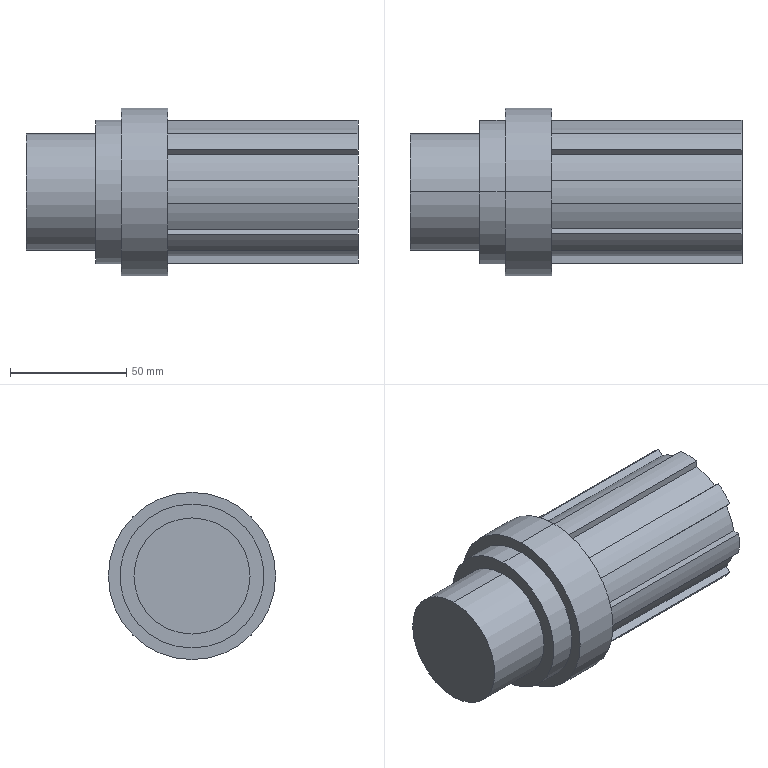Part | SolidWorks | features ICE 2, CirPattern 1, Revolution 1 | 1 solid | 44 faces | box 143 x 72 x 72 mm | volume 395287 mm3 | cylinder 23 | plane 21 | commonest cylinder face diameters 62 x11 56 x8 50 x2 72 x2
STEP:
#1=CARTESIAN_POINT('',(-30.,0.,25.));
#2=VERTEX_POINT('',#1);
#3=CARTESIAN_POINT('',(-30.,0.,-25.));
#4=VERTEX_POINT('',#3);
#5=CARTESIAN_POINT('',(-30.,0.,0.));
#6=DIRECTION('',(-1.,0.,0.));
#7=DIRECTION('',(0.,0.,1.));
#8=AXIS2_PLACEMENT_3D('',#5,#6,#7);
#9=CIRCLE('',#8,25.);
#10=EDGE_CURVE('',#2,#4,#9,.T.);
#11=ORIENTED_EDGE('',*,*,#10,.F.);
#12=CARTESIAN_POINT('',(0.,0.,25.));
#13=VERTEX_POINT('',#12);
#14=CARTESIAN_POINT('',(-30.,0.,25.));
#15=DIRECTION('',(1.,0.,0.));
#16=VECTOR('',#15,1000.);
#17=LINE('',#14,#16);
#18=EDGE_CURVE('',#2,#13,#17,.T.);
#19=ORIENTED_EDGE('',*,*,#18,.T.);
#20=CARTESIAN_POINT('',(0.,0.,-25.));
#21=VERTEX_POINT('',#20);
#22=CARTESIAN_POINT('',(0.,0.,0.));
#23=DIRECTION('',(-1.,0.,0.));
#24=DIRECTION('',(0.,0.,1.));
#25=AXIS2_PLACEMENT_3D('',#22,#23,#24);
#26=CIRCLE('',#25,25.);
#27=EDGE_CURVE('',#13,#21,#26,.T.);
#28=ORIENTED_EDGE('',*,*,#27,.T.);
#29=CARTESIAN_POINT('',(-30.,0.,-25.));
#30=DIRECTION('',(1.,0.,0.));
#31=VECTOR('',#30,1000.);
#32=LINE('',#29,#31);
#33=EDGE_CURVE('',#4,#21,#32,.T.);
#34=ORIENTED_EDGE('',*,*,#33,.F.);
#35=EDGE_LOOP('',(#11,#19,#28,#34));
#36=FACE_OUTER_BOUND('',#35,.T.);
#37=CARTESIAN_POINT('',(-30.,0.,0.));
#38=DIRECTION('',(1.,0.,0.));
#39=DIRECTION('',(0.,0.,-1.));
#40=AXIS2_PLACEMENT_3D('',#37,#38,#39);
#41=CYLINDRICAL_SURFACE('',#40,25.);
#42=ADVANCED_FACE('',(#36),#41,.T.);
#43=CARTESIAN_POINT('',(31.,0.,-31.));
#44=VERTEX_POINT('',#43);
#45=CARTESIAN_POINT('',(31.,-5.,-30.594));
#46=VERTEX_POINT('',#45);
#47=CARTESIAN_POINT('',(31.,0.,0.));
#48=DIRECTION('',(-1.,0.,0.));
#49=DIRECTION('',(0.,0.,-1.));
#50=AXIS2_PLACEMENT_3D('',#47,#48,#49);
#51=CIRCLE('',#50,31.);
#52=EDGE_CURVE('',#44,#46,#51,.T.);
#53=ORIENTED_EDGE('',*,*,#52,.F.);
#54=CARTESIAN_POINT('',(113.,0.,-31.));
#55=VERTEX_POINT('',#54);
#56=CARTESIAN_POINT('',(20.422,0.,-31.));
#57=DIRECTION('',(1.,0.,0.));
#58=VECTOR('',#57,1000.);
#59=LINE('',#56,#58);
#60=EDGE_CURVE('',#44,#55,#59,.T.);
#61=ORIENTED_EDGE('',*,*,#60,.T.);
#62=CARTESIAN_POINT('',(113.,-5.,-30.594));
#63=VERTEX_POINT('',#62);
#64=CARTESIAN_POINT('',(113.,0.,0.));
#65=DIRECTION('',(1.,0.,0.));
#66=DIRECTION('',(0.,-1.,0.));
#67=AXIS2_PLACEMENT_3D('',#64,#65,#66);
#68=CIRCLE('',#67,31.);
#69=EDGE_CURVE('',#63,#55,#68,.T.);
#70=ORIENTED_EDGE('',*,*,#69,.F.);
#71=CARTESIAN_POINT('',(20.422,-5.,-30.594));
#72=DIRECTION('',(1.,0.,0.));
#73=VECTOR('',#72,1000.);
#74=LINE('',#71,#73);
#75=EDGE_CURVE('',#46,#63,#74,.T.);
#76=ORIENTED_EDGE('',*,*,#75,.F.);
#77=EDGE_LOOP('',(#53,#61,#70,#76));
#78=FACE_OUTER_BOUND('',#77,.T.);
#79=CARTESIAN_POINT('',(20.422,0.,0.));
#80=DIRECTION('',(1.,0.,0.));
#81=DIRECTION('',(0.,0.,-1.));
#82=AXIS2_PLACEMENT_3D('',#79,#80,#81);
#83=CYLINDRICAL_SURFACE('',#82,31.);
#84=ADVANCED_FACE('',(#78),#83,.T.);
#85=CARTESIAN_POINT('',(11.,0.,-36.));
#86=VERTEX_POINT('',#85);
#87=CARTESIAN_POINT('',(11.,0.,36.));
#88=VERTEX_POINT('',#87);
#89=CARTESIAN_POINT('',(11.,0.,0.));
#90=DIRECTION('',(1.,0.,0.));
#91=DIRECTION('',(0.,0.,-1.));
#92=AXIS2_PLACEMENT_3D('',#89,#90,#91);
#93=CIRCLE('',#92,36.);
#94=EDGE_CURVE('',#86,#88,#93,.T.);
#95=ORIENTED_EDGE('',*,*,#94,.T.);
#96=CARTESIAN_POINT('',(31.,0.,36.));
#97=VERTEX_POINT('',#96);
#98=CARTESIAN_POINT('',(113.,0.,36.));
#99=DIRECTION('',(1.,0.,0.));
#100=VECTOR('',#99,1000.);
#101=LINE('',#98,#100);
#102=EDGE_CURVE('',#88,#97,#101,.T.);
#103=ORIENTED_EDGE('',*,*,#102,.T.);
#104=CARTESIAN_POINT('',(31.,0.,-36.));
#105=VERTEX_POINT('',#104);
#106=CARTESIAN_POINT('',(31.,0.,0.));
#107=DIRECTION('',(1.,0.,0.));
#108=DIRECTION('',(0.,0.,-1.));
#109=AXIS2_PLACEMENT_3D('',#106,#107,#108);
#110=CIRCLE('',#109,36.);
#111=EDGE_CURVE('',#105,#97,#110,.T.);
#112=ORIENTED_EDGE('',*,*,#111,.F.);
#113=CARTESIAN_POINT('',(113.,0.,-36.));
#114=DIRECTION('',(1.,0.,0.));
#115=VECTOR('',#114,1000.);
#116=LINE('',#113,#115);
#117=EDGE_CURVE('',#86,#105,#116,.T.);
#118=ORIENTED_EDGE('',*,*,#117,.F.);
#119=EDGE_LOOP('',(#95,#103,#112,#118));
#120=FACE_OUTER_BOUND('',#119,.T.);
#121=CARTESIAN_POINT('',(113.,0.,0.));
#122=DIRECTION('',(1.,0.,0.));
#123=DIRECTION('',(0.,0.,-1.));
#124=AXIS2_PLACEMENT_3D('',#121,#122,#123);
#125=CYLINDRICAL_SURFACE('',#124,36.);
#126=ADVANCED_FACE('',(#120),#125,.T.);
#127=CARTESIAN_POINT('',(0.,0.,-31.));
#128=VERTEX_POINT('',#127);
#129=CARTESIAN_POINT('',(0.,0.,31.));
#130=VERTEX_POINT('',#129);
#131=CARTESIAN_POINT('',(0.,0.,0.));
#132=DIRECTION('',(1.,0.,0.));
#133=DIRECTION('',(0.,0.,-1.));
#134=AXIS2_PLACEMENT_3D('',#131,#132,#133);
#135=CIRCLE('',#134,31.);
#136=EDGE_CURVE('',#128,#130,#135,.T.);
#137=ORIENTED_EDGE('',*,*,#136,.T.);
#138=CARTESIAN_POINT('',(11.,0.,31.));
#139=VERTEX_POINT('',#138);
#140=CARTESIAN_POINT('',(113.,0.,31.));
#141=DIRECTION('',(1.,0.,0.));
#142=VECTOR('',#141,1000.);
#143=LINE('',#140,#142);
#144=EDGE_CURVE('',#130,#139,#143,.T.);
#145=ORIENTED_EDGE('',*,*,#144,.T.);
#146=CARTESIAN_POINT('',(11.,0.,-31.));
#147=VERTEX_POINT('',#146);
#148=CARTESIAN_POINT('',(11.,0.,0.));
#149=DIRECTION('',(1.,0.,0.));
#150=DIRECTION('',(0.,0.,-1.));
#151=AXIS2_PLACEMENT_3D('',#148,#149,#150);
#152=CIRCLE('',#151,31.);
#153=EDGE_CURVE('',#147,#139,#152,.T.);
#154=ORIENTED_EDGE('',*,*,#153,.F.);
#155=CARTESIAN_POINT('',(113.,0.,-31.));
#156=DIRECTION('',(1.,0.,0.));
#157=VECTOR('',#156,1000.);
#158=LINE('',#155,#157);
#159=EDGE_CURVE('',#128,#147,#158,.T.);
#160=ORIENTED_EDGE('',*,*,#159,.F.);
#161=EDGE_LOOP('',(#137,#145,#154,#160));
#162=FACE_OUTER_BOUND('',#161,.T.);
#163=CARTESIAN_POINT('',(113.,0.,0.));
#164=DIRECTION('',(1.,0.,0.));
#165=DIRECTION('',(0.,0.,-1.));
#166=AXIS2_PLACEMENT_3D('',#163,#164,#165);
#167=CYLINDRICAL_SURFACE('',#166,31.);
#168=ADVANCED_FACE('',(#162),#167,.T.);
#169=CARTESIAN_POINT('',(31.,23.016,-15.945));
#170=VERTEX_POINT('',#169);
#171=CARTESIAN_POINT('',(113.,23.016,-15.945));
#172=VERTEX_POINT('',#171);
#173=CARTESIAN_POINT('',(17.956,23.016,-15.945));
#174=DIRECTION('',(1.,0.,0.));
#175=VECTOR('',#174,1000.);
#176=LINE('',#173,#175);
#177=EDGE_CURVE('',#170,#172,#176,.T.);
#178=ORIENTED_EDGE('',*,*,#177,.F.);
#179=CARTESIAN_POINT('',(31.,27.55,-5.));
#180=VERTEX_POINT('',#179);
#181=CARTESIAN_POINT('',(31.,0.,0.));
#182=DIRECTION('',(1.,0.,0.));
#183=DIRECTION('',(0.,0.,-1.));
#184=AXIS2_PLACEMENT_3D('',#181,#182,#183);
#185=CIRCLE('',#184,28.);
#186=EDGE_CURVE('',#170,#180,#185,.T.);
#187=ORIENTED_EDGE('',*,*,#186,.T.);
#188=CARTESIAN_POINT('',(113.,27.55,-5.));
#189=VERTEX_POINT('',#188);
#190=CARTESIAN_POINT('',(20.422,27.55,-5.));
#191=DIRECTION('',(1.,0.,0.));
#192=VECTOR('',#191,1000.);
#193=LINE('',#190,#192);
#194=EDGE_CURVE('',#180,#189,#193,.T.);
#195=ORIENTED_EDGE('',*,*,#194,.T.);
#196=CARTESIAN_POINT('',(113.,0.,0.));
#197=DIRECTION('',(1.,0.,0.));
#198=DIRECTION('',(0.,0.,-1.));
#199=AXIS2_PLACEMENT_3D('',#196,#197,#198);
#200=CIRCLE('',#199,28.);
#201=EDGE_CURVE('',#172,#189,#200,.T.);
#202=ORIENTED_EDGE('',*,*,#201,.F.);
#203=EDGE_LOOP('',(#178,#187,#195,#202));
#204=FACE_OUTER_BOUND('',#203,.T.);
#205=CARTESIAN_POINT('',(113.,0.,0.));
#206=DIRECTION('',(1.,0.,0.));
#207=DIRECTION('',(0.,0.,-1.));
#208=AXIS2_PLACEMENT_3D('',#205,#206,#207);
#209=CYLINDRICAL_SURFACE('',#208,28.);
#210=ADVANCED_FACE('',(#204),#209,.T.);
#211=CARTESIAN_POINT('',(31.,15.945,-23.016));
#212=VERTEX_POINT('',#211);
#213=CARTESIAN_POINT('',(113.,15.945,-23.016));
#214=VERTEX_POINT('',#213);
#215=CARTESIAN_POINT('',(17.956,15.945,-23.016));
#216=DIRECTION('',(1.,0.,0.));
#217=VECTOR('',#216,1000.);
#218=LINE('',#215,#217);
#219=EDGE_CURVE('',#212,#214,#218,.T.);
#220=ORIENTED_EDGE('',*,*,#219,.T.);
#221=CARTESIAN_POINT('',(113.,5.,-27.55));
#222=VERTEX_POINT('',#221);
#223=CARTESIAN_POINT('',(113.,0.,0.));
#224=DIRECTION('',(1.,0.,0.));
#225=DIRECTION('',(0.,0.,-1.));
#226=AXIS2_PLACEMENT_3D('',#223,#224,#225);
#227=CIRCLE('',#226,28.);
#228=EDGE_CURVE('',#222,#214,#227,.T.);
#229=ORIENTED_EDGE('',*,*,#228,.F.);
#230=CARTESIAN_POINT('',(31.,5.,-27.55));
#231=VERTEX_POINT('',#230);
#232=CARTESIAN_POINT('',(20.422,5.,-27.55));
#233=DIRECTION('',(1.,0.,0.));
#234=VECTOR('',#233,1000.);
#235=LINE('',#232,#234);
#236=EDGE_CURVE('',#231,#222,#235,.T.);
#237=ORIENTED_EDGE('',*,*,#236,.F.);
#238=CARTESIAN_POINT('',(31.,0.,0.));
#239=DIRECTION('',(1.,0.,0.));
#240=DIRECTION('',(0.,0.,-1.));
#241=AXIS2_PLACEMENT_3D('',#238,#239,#240);
#242=CIRCLE('',#241,28.);
#243=EDGE_CURVE('',#231,#212,#242,.T.);
#244=ORIENTED_EDGE('',*,*,#243,.T.);
#245=EDGE_LOOP('',(#220,#229,#237,#244));
#246=FACE_OUTER_BOUND('',#245,.T.);
#247=CARTESIAN_POINT('',(113.,0.,0.));
#248=DIRECTION('',(1.,0.,0.));
#249=DIRECTION('',(0.,0.,-1.));
#250=AXIS2_PLACEMENT_3D('',#247,#248,#249);
#251=CYLINDRICAL_SURFACE('',#250,28.);
#252=ADVANCED_FACE('',(#246),#251,.T.);
#253=CARTESIAN_POINT('',(31.,-5.,-27.55));
#254=VERTEX_POINT('',#253);
#255=CARTESIAN_POINT('',(113.,-5.,-27.55));
#256=VERTEX_POINT('',#255);
#257=CARTESIAN_POINT('',(20.422,-5.,-27.55));
#258=DIRECTION('',(1.,0.,0.));
#259=VECTOR('',#258,1000.);
#260=LINE('',#257,#259);
#261=EDGE_CURVE('',#254,#256,#260,.T.);
#262=ORIENTED_EDGE('',*,*,#261,.T.);
#263=CARTESIAN_POINT('',(113.,-15.945,-23.016));
#264=VERTEX_POINT('',#263);
#265=CARTESIAN_POINT('',(113.,0.,0.));
#266=DIRECTION('',(1.,0.,0.));
#267=DIRECTION('',(0.,0.,-1.));
#268=AXIS2_PLACEMENT_3D('',#265,#266,#267);
#269=CIRCLE('',#268,28.);
#270=EDGE_CURVE('',#264,#256,#269,.T.);
#271=ORIENTED_EDGE('',*,*,#270,.F.);
#272=CARTESIAN_POINT('',(31.,-15.945,-23.016));
#273=VERTEX_POINT('',#272);
#274=CARTESIAN_POINT('',(17.956,-15.945,-23.016));
#275=DIRECTION('',(1.,0.,0.));
#276=VECTOR('',#275,1000.);
#277=LINE('',#274,#276);
#278=EDGE_CURVE('',#273,#264,#277,.T.);
#279=ORIENTED_EDGE('',*,*,#278,.F.);
#280=CARTESIAN_POINT('',(31.,0.,0.));
#281=DIRECTION('',(1.,0.,0.));
#282=DIRECTION('',(0.,0.,-1.));
#283=AXIS2_PLACEMENT_3D('',#280,#281,#282);
#284=CIRCLE('',#283,28.);
#285=EDGE_CURVE('',#273,#254,#284,.T.);
#286=ORIENTED_EDGE('',*,*,#285,.T.);
#287=EDGE_LOOP('',(#262,#271,#279,#286));
#288=FACE_OUTER_BOUND('',#287,.T.);
#289=CARTESIAN_POINT('',(113.,0.,0.));
#290=DIRECTION('',(1.,0.,0.));
#291=DIRECTION('',(0.,0.,-1.));
#292=AXIS2_PLACEMENT_3D('',#289,#290,#291);
#293=CYLINDRICAL_SURFACE('',#292,28.);
#294=ADVANCED_FACE('',(#288),#293,.T.);
#295=CARTESIAN_POINT('',(31.,-23.016,-15.945));
#296=VERTEX_POINT('',#295);
#297=CARTESIAN_POINT('',(113.,-23.016,-15.945));
#298=VERTEX_POINT('',#297);
#299=CARTESIAN_POINT('',(17.956,-23.016,-15.945));
#300=DIRECTION('',(1.,0.,0.));
#301=VECTOR('',#300,1000.);
#302=LINE('',#299,#301);
#303=EDGE_CURVE('',#296,#298,#302,.T.);
#304=ORIENTED_EDGE('',*,*,#303,.T.);
#305=CARTESIAN_POINT('',(113.,-27.55,-5.));
#306=VERTEX_POINT('',#305);
#307=CARTESIAN_POINT('',(113.,0.,0.));
#308=DIRECTION('',(1.,0.,0.));
#309=DIRECTION('',(0.,0.,-1.));
#310=AXIS2_PLACEMENT_3D('',#307,#308,#309);
#311=CIRCLE('',#310,28.);
#312=EDGE_CURVE('',#306,#298,#311,.T.);
#313=ORIENTED_EDGE('',*,*,#312,.F.);
#314=CARTESIAN_POINT('',(31.,-27.55,-5.));
#315=VERTEX_POINT('',#314);
#316=CARTESIAN_POINT('',(20.422,-27.55,-5.));
#317=DIRECTION('',(1.,0.,0.));
#318=VECTOR('',#317,1000.);
#319=LINE('',#316,#318);
#320=EDGE_CURVE('',#315,#306,#319,.T.);
#321=ORIENTED_EDGE('',*,*,#320,.F.);
#322=CARTESIAN_POINT('',(31.,0.,0.));
#323=DIRECTION('',(1.,0.,0.));
#324=DIRECTION('',(0.,0.,-1.));
#325=AXIS2_PLACEMENT_3D('',#322,#323,#324);
#326=CIRCLE('',#325,28.);
#327=EDGE_CURVE('',#315,#296,#326,.T.);
#328=ORIENTED_EDGE('',*,*,#327,.T.);
#329=EDGE_LOOP('',(#304,#313,#321,#328));
#330=FACE_OUTER_BOUND('',#329,.T.);
#331=CARTESIAN_POINT('',(113.,0.,0.));
#332=DIRECTION('',(1.,0.,0.));
#333=DIRECTION('',(0.,0.,-1.));
#334=AXIS2_PLACEMENT_3D('',#331,#332,#333);
#335=CYLINDRICAL_SURFACE('',#334,28.);
#336=ADVANCED_FACE('',(#330),#335,.T.);
#337=CARTESIAN_POINT('',(31.,-27.55,5.));
#338=VERTEX_POINT('',#337);
#339=CARTESIAN_POINT('',(113.,-27.55,5.));
#340=VERTEX_POINT('',#339);
#341=CARTESIAN_POINT('',(20.422,-27.55,5.));
#342=DIRECTION('',(1.,0.,0.));
#343=VECTOR('',#342,1000.);
#344=LINE('',#341,#343);
#345=EDGE_CURVE('',#338,#340,#344,.T.);
#346=ORIENTED_EDGE('',*,*,#345,.T.);
#347=CARTESIAN_POINT('',(113.,-23.016,15.945));
#348=VERTEX_POINT('',#347);
#349=CARTESIAN_POINT('',(113.,0.,0.));
#350=DIRECTION('',(1.,0.,0.));
#351=DIRECTION('',(0.,0.,-1.));
#352=AXIS2_PLACEMENT_3D('',#349,#350,#351);
#353=CIRCLE('',#352,28.);
#354=EDGE_CURVE('',#348,#340,#353,.T.);
#355=ORIENTED_EDGE('',*,*,#354,.F.);
#356=CARTESIAN_POINT('',(31.,-23.016,15.945));
#357=VERTEX_POINT('',#356);
#358=CARTESIAN_POINT('',(17.956,-23.016,15.945));
#359=DIRECTION('',(1.,0.,0.));
#360=VECTOR('',#359,1000.);
#361=LINE('',#358,#360);
#362=EDGE_CURVE('',#357,#348,#361,.T.);
#363=ORIENTED_EDGE('',*,*,#362,.F.);
#364=CARTESIAN_POINT('',(31.,0.,0.));
#365=DIRECTION('',(1.,0.,0.));
#366=DIRECTION('',(0.,0.,-1.));
#367=AXIS2_PLACEMENT_3D('',#364,#365,#366);
#368=CIRCLE('',#367,28.);
#369=EDGE_CURVE('',#357,#338,#368,.T.);
#370=ORIENTED_EDGE('',*,*,#369,.T.);
#371=EDGE_LOOP('',(#346,#355,#363,#370));
#372=FACE_OUTER_BOUND('',#371,.T.);
#373=CARTESIAN_POINT('',(113.,0.,0.));
#374=DIRECTION('',(1.,0.,0.));
#375=DIRECTION('',(0.,0.,-1.));
#376=AXIS2_PLACEMENT_3D('',#373,#374,#375);
#377=CYLINDRICAL_SURFACE('',#376,28.);
#378=ADVANCED_FACE('',(#372),#377,.T.);
#379=CARTESIAN_POINT('',(31.,-15.945,23.016));
#380=VERTEX_POINT('',#379);
#381=CARTESIAN_POINT('',(113.,-15.945,23.016));
#382=VERTEX_POINT('',#381);
#383=CARTESIAN_POINT('',(17.956,-15.945,23.016));
#384=DIRECTION('',(1.,0.,0.));
#385=VECTOR('',#384,1000.);
#386=LINE('',#383,#385);
#387=EDGE_CURVE('',#380,#382,#386,.T.);
#388=ORIENTED_EDGE('',*,*,#387,.T.);
#389=CARTESIAN_POINT('',(113.,-5.,27.55));
#390=VERTEX_POINT('',#389);
#391=CARTESIAN_POINT('',(113.,0.,0.));
#392=DIRECTION('',(1.,0.,0.));
#393=DIRECTION('',(0.,0.,-1.));
#394=AXIS2_PLACEMENT_3D('',#391,#392,#393);
#395=CIRCLE('',#394,28.);
#396=EDGE_CURVE('',#390,#382,#395,.T.);
#397=ORIENTED_EDGE('',*,*,#396,.F.);
#398=CARTESIAN_POINT('',(31.,-5.,27.55));
#399=VERTEX_POINT('',#398);
#400=CARTESIAN_POINT('',(20.422,-5.,27.55));
#401=DIRECTION('',(1.,0.,0.));
#402=VECTOR('',#401,1000.);
#403=LINE('',#400,#402);
#404=EDGE_CURVE('',#399,#390,#403,.T.);
#405=ORIENTED_EDGE('',*,*,#404,.F.);
#406=CARTESIAN_POINT('',(31.,0.,0.));
#407=DIRECTION('',(1.,0.,0.));
#408=DIRECTION('',(0.,0.,-1.));
#409=AXIS2_PLACEMENT_3D('',#406,#407,#408);
#410=CIRCLE('',#409,28.);
#411=EDGE_CURVE('',#399,#380,#410,.T.);
#412=ORIENTED_EDGE('',*,*,#411,.T.);
#413=EDGE_LOOP('',(#388,#397,#405,#412));
#414=FACE_OUTER_BOUND('',#413,.T.);
#415=CARTESIAN_POINT('',(113.,0.,0.));
#416=DIRECTION('',(1.,0.,0.));
#417=DIRECTION('',(0.,0.,-1.));
#418=AXIS2_PLACEMENT_3D('',#415,#416,#417);
#419=CYLINDRICAL_SURFACE('',#418,28.);
#420=ADVANCED_FACE('',(#414),#419,.T.);
#421=CARTESIAN_POINT('',(31.,5.,27.55));
#422=VERTEX_POINT('',#421);
#423=CARTESIAN_POINT('',(113.,5.,27.55));
#424=VERTEX_POINT('',#423);
#425=CARTESIAN_POINT('',(20.422,5.,27.55));
#426=DIRECTION('',(1.,0.,0.));
#427=VECTOR('',#426,1000.);
#428=LINE('',#425,#427);
#429=EDGE_CURVE('',#422,#424,#428,.T.);
#430=ORIENTED_EDGE('',*,*,#429,.T.);
#431=CARTESIAN_POINT('',(113.,15.945,23.016));
#432=VERTEX_POINT('',#431);
#433=CARTESIAN_POINT('',(113.,0.,0.));
#434=DIRECTION('',(1.,0.,0.));
#435=DIRECTION('',(0.,0.,-1.));
#436=AXIS2_PLACEMENT_3D('',#433,#434,#435);
#437=CIRCLE('',#436,28.);
#438=EDGE_CURVE('',#432,#424,#437,.T.);
#439=ORIENTED_EDGE('',*,*,#438,.F.);
#440=CARTESIAN_POINT('',(31.,15.945,23.016));
#441=VERTEX_POINT('',#440);
#442=CARTESIAN_POINT('',(17.956,15.945,23.016));
#443=DIRECTION('',(1.,0.,0.));
#444=VECTOR('',#443,1000.);
#445=LINE('',#442,#444);
#446=EDGE_CURVE('',#441,#432,#445,.T.);
#447=ORIENTED_EDGE('',*,*,#446,.F.);
#448=CARTESIAN_POINT('',(31.,0.,0.));
#449=DIRECTION('',(1.,0.,0.));
#450=DIRECTION('',(0.,0.,-1.));
#451=AXIS2_PLACEMENT_3D('',#448,#449,#450);
#452=CIRCLE('',#451,28.);
#453=EDGE_CURVE('',#441,#422,#452,.T.);
#454=ORIENTED_EDGE('',*,*,#453,.T.);
#455=EDGE_LOOP('',(#430,#439,#447,#454));
#456=FACE_OUTER_BOUND('',#455,.T.);
#457=CARTESIAN_POINT('',(113.,0.,0.));
#458=DIRECTION('',(1.,0.,0.));
#459=DIRECTION('',(0.,0.,-1.));
#460=AXIS2_PLACEMENT_3D('',#457,#458,#459);
#461=CYLINDRICAL_SURFACE('',#460,28.);
#462=ADVANCED_FACE('',(#456),#461,.T.);
#463=CARTESIAN_POINT('',(0.,0.,0.));
#464=DIRECTION('',(-1.,0.,0.));
#465=DIRECTION('',(0.,0.,1.));
#466=AXIS2_PLACEMENT_3D('',#463,#464,#465);
#467=CIRCLE('',#466,25.);
#468=EDGE_CURVE('',#21,#13,#467,.T.);
#469=ORIENTED_EDGE('',*,*,#468,.F.);
#470=ORIENTED_EDGE('',*,*,#27,.F.);
#471=EDGE_LOOP('',(#469,#470));
#472=FACE_BOUND('',#471,.T.);
#473=ORIENTED_EDGE('',*,*,#136,.F.);
#474=CARTESIAN_POINT('',(0.,0.,0.));
#475=DIRECTION('',(1.,0.,0.));
#476=DIRECTION('',(0.,0.,-1.));
#477=AXIS2_PLACEMENT_3D('',#474,#475,#476);
#478=CIRCLE('',#477,31.);
#479=EDGE_CURVE('',#130,#128,#478,.T.);
#480=ORIENTED_EDGE('',*,*,#479,.F.);
#481=EDGE_LOOP('',(#473,#480));
#482=FACE_OUTER_BOUND('',#481,.T.);
#483=CARTESIAN_POINT('',(0.,0.,0.));
#484=DIRECTION('',(-1.,0.,0.));
#485=DIRECTION('',(0.,0.,1.));
#486=AXIS2_PLACEMENT_3D('',#483,#484,#485);
#487=PLANE('',#486);
#488=ADVANCED_FACE('',(#472,#482),#487,.T.);
#489=ORIENTED_EDGE('',*,*,#144,.F.);
#490=ORIENTED_EDGE('',*,*,#479,.T.);
#491=ORIENTED_EDGE('',*,*,#159,.T.);
#492=CARTESIAN_POINT('',(11.,0.,0.));
#493=DIRECTION('',(1.,0.,0.));
#494=DIRECTION('',(0.,0.,-1.));
#495=AXIS2_PLACEMENT_3D('',#492,#493,#494);
#496=CIRCLE('',#495,31.);
#497=EDGE_CURVE('',#139,#147,#496,.T.);
#498=ORIENTED_EDGE('',*,*,#497,.F.);
#499=EDGE_LOOP('',(#489,#490,#491,#498));
#500=FACE_OUTER_BOUND('',#499,.T.);
#501=CARTESIAN_POINT('',(113.,0.,0.));
#502=DIRECTION('',(1.,0.,0.));
#503=DIRECTION('',(0.,0.,-1.));
#504=AXIS2_PLACEMENT_3D('',#501,#502,#503);
#505=CYLINDRICAL_SURFACE('',#504,31.);
#506=ADVANCED_FACE('',(#500),#505,.T.);
#507=ORIENTED_EDGE('',*,*,#153,.T.);
#508=ORIENTED_EDGE('',*,*,#497,.T.);
#509=EDGE_LOOP('',(#507,#508));
#510=FACE_BOUND('',#509,.T.);
#511=ORIENTED_EDGE('',*,*,#94,.F.);
#512=CARTESIAN_POINT('',(11.,0.,0.));
#513=DIRECTION('',(1.,0.,0.));
#514=DIRECTION('',(0.,0.,-1.));
#515=AXIS2_PLACEMENT_3D('',#512,#513,#514);
#516=CIRCLE('',#515,36.);
#517=EDGE_CURVE('',#88,#86,#516,.T.);
#518=ORIENTED_EDGE('',*,*,#517,.F.);
#519=EDGE_LOOP('',(#511,#518));
#520=FACE_OUTER_BOUND('',#519,.T.);
#521=CARTESIAN_POINT('',(11.,0.,-31.));
#522=DIRECTION('',(-1.,0.,0.));
#523=DIRECTION('',(0.,0.,1.));
#524=AXIS2_PLACEMENT_3D('',#521,#522,#523);
#525=PLANE('',#524);
#526=ADVANCED_FACE('',(#510,#520),#525,.T.);
#527=ORIENTED_EDGE('',*,*,#102,.F.);
#528=ORIENTED_EDGE('',*,*,#517,.T.);
#529=ORIENTED_EDGE('',*,*,#117,.T.);
#530=CARTESIAN_POINT('',(31.,0.,0.));
#531=DIRECTION('',(1.,0.,0.));
#532=DIRECTION('',(0.,0.,-1.));
#533=AXIS2_PLACEMENT_3D('',#530,#531,#532);
#534=CIRCLE('',#533,36.);
#535=EDGE_CURVE('',#97,#105,#534,.T.);
#536=ORIENTED_EDGE('',*,*,#535,.F.);
#537=EDGE_LOOP('',(#527,#528,#529,#536));
#538=FACE_OUTER_BOUND('',#537,.T.);
#539=CARTESIAN_POINT('',(113.,0.,0.));
#540=DIRECTION('',(1.,0.,0.));
#541=DIRECTION('',(0.,0.,-1.));
#542=AXIS2_PLACEMENT_3D('',#539,#540,#541);
#543=CYLINDRICAL_SURFACE('',#542,36.);
#544=ADVANCED_FACE('',(#538),#543,.T.);
#545=CARTESIAN_POINT('',(31.,25.169,-18.098));
#546=VERTEX_POINT('',#545);
#547=CARTESIAN_POINT('',(31.,25.169,-18.098));
#548=DIRECTION('',(0.,0.7071,-0.7071));
#549=VECTOR('',#548,1000.);
#550=LINE('',#547,#549);
#551=EDGE_CURVE('',#170,#546,#550,.T.);
#552=ORIENTED_EDGE('',*,*,#551,.T.);
#553=CARTESIAN_POINT('',(31.,18.098,-25.169));
#554=VERTEX_POINT('',#553);
#555=CARTESIAN_POINT('',(31.,0.,0.));
#556=DIRECTION('',(-1.,0.,0.));
#557=DIRECTION('',(0.,0.,-1.));
#558=AXIS2_PLACEMENT_3D('',#555,#556,#557);
#559=CIRCLE('',#558,31.);
#560=EDGE_CURVE('',#546,#554,#559,.T.);
#561=ORIENTED_EDGE('',*,*,#560,.T.);
#562=CARTESIAN_POINT('',(31.,18.098,-25.169));
#563=DIRECTION('',(0.,-0.7071,0.7071));
#564=VECTOR('',#563,1000.);
#565=LINE('',#562,#564);
#566=EDGE_CURVE('',#554,#212,#565,.T.);
#567=ORIENTED_EDGE('',*,*,#566,.T.);
#568=ORIENTED_EDGE('',*,*,#243,.F.);
#569=CARTESIAN_POINT('',(31.,5.,-30.594));
#570=VERTEX_POINT('',#569);
#571=CARTESIAN_POINT('',(31.,5.,-30.594));
#572=DIRECTION('',(0.,0.,-1.));
#573=VECTOR('',#572,1000.);
#574=LINE('',#571,#573);
#575=EDGE_CURVE('',#231,#570,#574,.T.);
#576=ORIENTED_EDGE('',*,*,#575,.T.);
#577=CARTESIAN_POINT('',(31.,0.,0.));
#578=DIRECTION('',(-1.,0.,0.));
#579=DIRECTION('',(0.,0.,-1.));
#580=AXIS2_PLACEMENT_3D('',#577,#578,#579);
#581=CIRCLE('',#580,31.);
#582=EDGE_CURVE('',#570,#44,#581,.T.);
#583=ORIENTED_EDGE('',*,*,#582,.T.);
#584=ORIENTED_EDGE('',*,*,#52,.T.);
#585=CARTESIAN_POINT('',(31.,-5.,-30.594));
#586=DIRECTION('',(0.,0.,1.));
#587=VECTOR('',#586,1000.);
#588=LINE('',#585,#587);
#589=EDGE_CURVE('',#46,#254,#588,.T.);
#590=ORIENTED_EDGE('',*,*,#589,.T.);
#591=ORIENTED_EDGE('',*,*,#285,.F.);
#592=CARTESIAN_POINT('',(31.,-18.098,-25.169));
#593=VERTEX_POINT('',#592);
#594=CARTESIAN_POINT('',(31.,-18.098,-25.169));
#595=DIRECTION('',(0.,-0.7071,-0.7071));
#596=VECTOR('',#595,1000.);
#597=LINE('',#594,#596);
#598=EDGE_CURVE('',#273,#593,#597,.T.);
#599=ORIENTED_EDGE('',*,*,#598,.T.);
#600=CARTESIAN_POINT('',(31.,-25.169,-18.098));
#601=VERTEX_POINT('',#600);
#602=CARTESIAN_POINT('',(31.,0.,0.));
#603=DIRECTION('',(-1.,0.,0.));
#604=DIRECTION('',(0.,0.,-1.));
#605=AXIS2_PLACEMENT_3D('',#602,#603,#604);
#606=CIRCLE('',#605,31.);
#607=EDGE_CURVE('',#593,#601,#606,.T.);
#608=ORIENTED_EDGE('',*,*,#607,.T.);
#609=CARTESIAN_POINT('',(31.,-25.169,-18.098));
#610=DIRECTION('',(0.,0.7071,0.7071));
#611=VECTOR('',#610,1000.);
#612=LINE('',#609,#611);
#613=EDGE_CURVE('',#601,#296,#612,.T.);
#614=ORIENTED_EDGE('',*,*,#613,.T.);
#615=ORIENTED_EDGE('',*,*,#327,.F.);
#616=CARTESIAN_POINT('',(31.,-30.594,-5.));
#617=VERTEX_POINT('',#616);
#618=CARTESIAN_POINT('',(31.,-30.594,-5.));
#619=DIRECTION('',(0.,-1.,0.));
#620=VECTOR('',#619,1000.);
#621=LINE('',#618,#620);
#622=EDGE_CURVE('',#315,#617,#621,.T.);
#623=ORIENTED_EDGE('',*,*,#622,.T.);
#624=CARTESIAN_POINT('',(31.,-30.594,5.));
#625=VERTEX_POINT('',#624);
#626=CARTESIAN_POINT('',(31.,0.,0.));
#627=DIRECTION('',(-1.,0.,0.));
#628=DIRECTION('',(0.,0.,-1.));
#629=AXIS2_PLACEMENT_3D('',#626,#627,#628);
#630=CIRCLE('',#629,31.);
#631=EDGE_CURVE('',#617,#625,#630,.T.);
#632=ORIENTED_EDGE('',*,*,#631,.T.);
#633=CARTESIAN_POINT('',(31.,-30.594,5.));
#634=DIRECTION('',(0.,1.,0.));
#635=VECTOR('',#634,1000.);
#636=LINE('',#633,#635);
#637=EDGE_CURVE('',#625,#338,#636,.T.);
#638=ORIENTED_EDGE('',*,*,#637,.T.);
#639=ORIENTED_EDGE('',*,*,#369,.F.);
#640=CARTESIAN_POINT('',(31.,-25.169,18.098));
#641=VERTEX_POINT('',#640);
#642=CARTESIAN_POINT('',(31.,-25.169,18.098));
#643=DIRECTION('',(0.,-0.7071,0.7071));
#644=VECTOR('',#643,1000.);
#645=LINE('',#642,#644);
#646=EDGE_CURVE('',#357,#641,#645,.T.);
#647=ORIENTED_EDGE('',*,*,#646,.T.);
#648=CARTESIAN_POINT('',(31.,-18.098,25.169));
#649=VERTEX_POINT('',#648);
#650=CARTESIAN_POINT('',(31.,0.,0.));
#651=DIRECTION('',(-1.,0.,0.));
#652=DIRECTION('',(0.,0.,-1.));
#653=AXIS2_PLACEMENT_3D('',#650,#651,#652);
#654=CIRCLE('',#653,31.);
#655=EDGE_CURVE('',#641,#649,#654,.T.);
#656=ORIENTED_EDGE('',*,*,#655,.T.);
#657=CARTESIAN_POINT('',(31.,-18.098,25.169));
#658=DIRECTION('',(0.,0.7071,-0.7071));
#659=VECTOR('',#658,1000.);
#660=LINE('',#657,#659);
#661=EDGE_CURVE('',#649,#380,#660,.T.);
#662=ORIENTED_EDGE('',*,*,#661,.T.);
#663=ORIENTED_EDGE('',*,*,#411,.F.);
#664=CARTESIAN_POINT('',(31.,-5.,30.594));
#665=VERTEX_POINT('',#664);
#666=CARTESIAN_POINT('',(31.,-5.,30.594));
#667=DIRECTION('',(0.,0.,1.));
#668=VECTOR('',#667,1000.);
#669=LINE('',#666,#668);
#670=EDGE_CURVE('',#399,#665,#669,.T.);
#671=ORIENTED_EDGE('',*,*,#670,.T.);
#672=CARTESIAN_POINT('',(31.,5.,30.594));
#673=VERTEX_POINT('',#672);
#674=CARTESIAN_POINT('',(31.,0.,0.));
#675=DIRECTION('',(-1.,0.,0.));
#676=DIRECTION('',(0.,0.,-1.));
#677=AXIS2_PLACEMENT_3D('',#674,#675,#676);
#678=CIRCLE('',#677,31.);
#679=EDGE_CURVE('',#665,#673,#678,.T.);
#680=ORIENTED_EDGE('',*,*,#679,.T.);
#681=CARTESIAN_POINT('',(31.,5.,30.594));
#682=DIRECTION('',(0.,0.,-1.));
#683=VECTOR('',#682,1000.);
#684=LINE('',#681,#683);
#685=EDGE_CURVE('',#673,#422,#684,.T.);
#686=ORIENTED_EDGE('',*,*,#685,.T.);
#687=ORIENTED_EDGE('',*,*,#453,.F.);
#688=CARTESIAN_POINT('',(31.,18.098,25.169));
#689=VERTEX_POINT('',#688);
#690=CARTESIAN_POINT('',(31.,18.098,25.169));
#691=DIRECTION('',(0.,0.7071,0.7071));
#692=VECTOR('',#691,1000.);
#693=LINE('',#690,#692);
#694=EDGE_CURVE('',#441,#689,#693,.T.);
#695=ORIENTED_EDGE('',*,*,#694,.T.);
#696=CARTESIAN_POINT('',(31.,25.169,18.098));
#697=VERTEX_POINT('',#696);
#698=CARTESIAN_POINT('',(31.,0.,0.));
#699=DIRECTION('',(-1.,0.,0.));
#700=DIRECTION('',(0.,0.,-1.));
#701=AXIS2_PLACEMENT_3D('',#698,#699,#700);
#702=CIRCLE('',#701,31.);
#703=EDGE_CURVE('',#689,#697,#702,.T.);
#704=ORIENTED_EDGE('',*,*,#703,.T.);
#705=CARTESIAN_POINT('',(31.,23.016,15.945));
#706=VERTEX_POINT('',#705);
#707=CARTESIAN_POINT('',(31.,25.169,18.098));
#708=DIRECTION('',(0.,-0.7071,-0.7071));
#709=VECTOR('',#708,1000.);
#710=LINE('',#707,#709);
#711=EDGE_CURVE('',#697,#706,#710,.T.);
#712=ORIENTED_EDGE('',*,*,#711,.T.);
#713=CARTESIAN_POINT('',(31.,27.55,5.));
#714=VERTEX_POINT('',#713);
#715=CARTESIAN_POINT('',(31.,0.,0.));
#716=DIRECTION('',(1.,0.,0.));
#717=DIRECTION('',(0.,0.,-1.));
#718=AXIS2_PLACEMENT_3D('',#715,#716,#717);
#719=CIRCLE('',#718,28.);
#720=EDGE_CURVE('',#714,#706,#719,.T.);
#721=ORIENTED_EDGE('',*,*,#720,.F.);
#722=CARTESIAN_POINT('',(31.,30.594,5.));
#723=VERTEX_POINT('',#722);
#724=CARTESIAN_POINT('',(31.,30.594,5.));
#725=DIRECTION('',(0.,1.,0.));
#726=VECTOR('',#725,1000.);
#727=LINE('',#724,#726);
#728=EDGE_CURVE('',#714,#723,#727,.T.);
#729=ORIENTED_EDGE('',*,*,#728,.T.);
#730=CARTESIAN_POINT('',(31.,30.594,-5.));
#731=VERTEX_POINT('',#730);
#732=CARTESIAN_POINT('',(31.,0.,0.));
#733=DIRECTION('',(-1.,0.,0.));
#734=DIRECTION('',(0.,0.,-1.));
#735=AXIS2_PLACEMENT_3D('',#732,#733,#734);
#736=CIRCLE('',#735,31.);
#737=EDGE_CURVE('',#723,#731,#736,.T.);
#738=ORIENTED_EDGE('',*,*,#737,.T.);
#739=CARTESIAN_POINT('',(31.,30.594,-5.));
#740=DIRECTION('',(0.,-1.,0.));
#741=VECTOR('',#740,1000.);
#742=LINE('',#739,#741);
#743=EDGE_CURVE('',#731,#180,#742,.T.);
#744=ORIENTED_EDGE('',*,*,#743,.T.);
#745=ORIENTED_EDGE('',*,*,#186,.F.);
#746=EDGE_LOOP('',(#552,#561,#567,#568,#576,#583,#584,#590,#591,#599,#608,#614,#615,#623,#632,#638,#639,#647,#656,#662,#663,#671,#680,#686,#687,#695,#704,#712,#721,#729,#738,#744,#745));
#747=FACE_BOUND('',#746,.T.);
#748=ORIENTED_EDGE('',*,*,#111,.T.);
#749=ORIENTED_EDGE('',*,*,#535,.T.);
#750=EDGE_LOOP('',(#748,#749));
#751=FACE_OUTER_BOUND('',#750,.T.);
#752=CARTESIAN_POINT('',(31.,0.,-36.));
#753=DIRECTION('',(1.,0.,0.));
#754=DIRECTION('',(0.,0.,-1.));
#755=AXIS2_PLACEMENT_3D('',#752,#753,#754);
#756=PLANE('',#755);
#757=ADVANCED_FACE('',(#747,#751),#756,.T.);
#758=CARTESIAN_POINT('',(113.,23.016,15.945));
#759=VERTEX_POINT('',#758);
#760=CARTESIAN_POINT('',(17.956,23.016,15.945));
#761=DIRECTION('',(1.,0.,0.));
#762=VECTOR('',#761,1000.);
#763=LINE('',#760,#762);
#764=EDGE_CURVE('',#706,#759,#763,.T.);
#765=ORIENTED_EDGE('',*,*,#764,.T.);
#766=CARTESIAN_POINT('',(113.,27.55,5.));
#767=VERTEX_POINT('',#766);
#768=CARTESIAN_POINT('',(113.,0.,0.));
#769=DIRECTION('',(1.,0.,0.));
#770=DIRECTION('',(0.,0.,-1.));
#771=AXIS2_PLACEMENT_3D('',#768,#769,#770);
#772=CIRCLE('',#771,28.);
#773=EDGE_CURVE('',#767,#759,#772,.T.);
#774=ORIENTED_EDGE('',*,*,#773,.F.);
#775=CARTESIAN_POINT('',(20.422,27.55,5.));
#776=DIRECTION('',(1.,0.,0.));
#777=VECTOR('',#776,1000.);
#778=LINE('',#775,#777);
#779=EDGE_CURVE('',#714,#767,#778,.T.);
#780=ORIENTED_EDGE('',*,*,#779,.F.);
#781=ORIENTED_EDGE('',*,*,#720,.T.);
#782=EDGE_LOOP('',(#765,#774,#780,#781));
#783=FACE_OUTER_BOUND('',#782,.T.);
#784=CARTESIAN_POINT('',(113.,0.,0.));
#785=DIRECTION('',(1.,0.,0.));
#786=DIRECTION('',(0.,0.,-1.));
#787=AXIS2_PLACEMENT_3D('',#784,#785,#786);
#788=CYLINDRICAL_SURFACE('',#787,28.);
#789=ADVANCED_FACE('',(#783),#788,.T.);
#790=ORIENTED_EDGE('',*,*,#773,.T.);
#791=CARTESIAN_POINT('',(113.,25.169,18.098));
#792=VERTEX_POINT('',#791);
#793=CARTESIAN_POINT('',(113.,25.169,18.098));
#794=DIRECTION('',(0.,0.7071,0.7071));
#795=VECTOR('',#794,1000.);
#796=LINE('',#793,#795);
#797=EDGE_CURVE('',#759,#792,#796,.T.);
#798=ORIENTED_EDGE('',*,*,#797,.T.);
#799=CARTESIAN_POINT('',(113.,18.098,25.169));
#800=VERTEX_POINT('',#799);
#801=CARTESIAN_POINT('',(113.,0.,0.));
#802=DIRECTION('',(1.,0.,0.));
#803=DIRECTION('',(0.,0.7071,-0.7071));
#804=AXIS2_PLACEMENT_3D('',#801,#802,#803);
#805=CIRCLE('',#804,31.);
#806=EDGE_CURVE('',#792,#800,#805,.T.);
#807=ORIENTED_EDGE('',*,*,#806,.T.);
#808=CARTESIAN_POINT('',(113.,18.098,25.169));
#809=DIRECTION('',(0.,-0.7071,-0.7071));
#810=VECTOR('',#809,1000.);
#811=LINE('',#808,#810);
#812=EDGE_CURVE('',#800,#432,#811,.T.);
#813=ORIENTED_EDGE('',*,*,#812,.T.);
#814=ORIENTED_EDGE('',*,*,#438,.T.);
#815=CARTESIAN_POINT('',(113.,5.,30.594));
#816=VERTEX_POINT('',#815);
#817=CARTESIAN_POINT('',(113.,5.,30.594));
#818=DIRECTION('',(0.,0.,1.));
#819=VECTOR('',#818,1000.);
#820=LINE('',#817,#819);
#821=EDGE_CURVE('',#424,#816,#820,.T.);
#822=ORIENTED_EDGE('',*,*,#821,.T.);
#823=CARTESIAN_POINT('',(113.,-5.,30.594));
#824=VERTEX_POINT('',#823);
#825=CARTESIAN_POINT('',(113.,0.,0.));
#826=DIRECTION('',(1.,0.,0.));
#827=DIRECTION('',(0.,1.,0.));
#828=AXIS2_PLACEMENT_3D('',#825,#826,#827);
#829=CIRCLE('',#828,31.);
#830=EDGE_CURVE('',#816,#824,#829,.T.);
#831=ORIENTED_EDGE('',*,*,#830,.T.);
#832=CARTESIAN_POINT('',(113.,-5.,30.594));
#833=DIRECTION('',(0.,0.,-1.));
#834=VECTOR('',#833,1000.);
#835=LINE('',#832,#834);
#836=EDGE_CURVE('',#824,#390,#835,.T.);
#837=ORIENTED_EDGE('',*,*,#836,.T.);
#838=ORIENTED_EDGE('',*,*,#396,.T.);
#839=CARTESIAN_POINT('',(113.,-18.098,25.169));
#840=VERTEX_POINT('',#839);
#841=CARTESIAN_POINT('',(113.,-18.098,25.169));
#842=DIRECTION('',(0.,-0.7071,0.7071));
#843=VECTOR('',#842,1000.);
#844=LINE('',#841,#843);
#845=EDGE_CURVE('',#382,#840,#844,.T.);
#846=ORIENTED_EDGE('',*,*,#845,.T.);
#847=CARTESIAN_POINT('',(113.,-25.169,18.098));
#848=VERTEX_POINT('',#847);
#849=CARTESIAN_POINT('',(113.,0.,0.));
#850=DIRECTION('',(1.,0.,0.));
#851=DIRECTION('',(0.,0.7071,0.7071));
#852=AXIS2_PLACEMENT_3D('',#849,#850,#851);
#853=CIRCLE('',#852,31.);
#854=EDGE_CURVE('',#840,#848,#853,.T.);
#855=ORIENTED_EDGE('',*,*,#854,.T.);
#856=CARTESIAN_POINT('',(113.,-25.169,18.098));
#857=DIRECTION('',(0.,0.7071,-0.7071));
#858=VECTOR('',#857,1000.);
#859=LINE('',#856,#858);
#860=EDGE_CURVE('',#848,#348,#859,.T.);
#861=ORIENTED_EDGE('',*,*,#860,.T.);
#862=ORIENTED_EDGE('',*,*,#354,.T.);
#863=CARTESIAN_POINT('',(113.,-30.594,5.));
#864=VERTEX_POINT('',#863);
#865=CARTESIAN_POINT('',(113.,-30.594,5.));
#866=DIRECTION('',(0.,-1.,0.));
#867=VECTOR('',#866,1000.);
#868=LINE('',#865,#867);
#869=EDGE_CURVE('',#340,#864,#868,.T.);
#870=ORIENTED_EDGE('',*,*,#869,.T.);
#871=CARTESIAN_POINT('',(113.,-30.594,-5.));
#872=VERTEX_POINT('',#871);
#873=CARTESIAN_POINT('',(113.,0.,0.));
#874=DIRECTION('',(1.,0.,0.));
#875=DIRECTION('',(0.,0.,1.));
#876=AXIS2_PLACEMENT_3D('',#873,#874,#875);
#877=CIRCLE('',#876,31.);
#878=EDGE_CURVE('',#864,#872,#877,.T.);
#879=ORIENTED_EDGE('',*,*,#878,.T.);
#880=CARTESIAN_POINT('',(113.,-30.594,-5.));
#881=DIRECTION('',(0.,1.,0.));
#882=VECTOR('',#881,1000.);
#883=LINE('',#880,#882);
#884=EDGE_CURVE('',#872,#306,#883,.T.);
#885=ORIENTED_EDGE('',*,*,#884,.T.);
#886=ORIENTED_EDGE('',*,*,#312,.T.);
#887=CARTESIAN_POINT('',(113.,-25.169,-18.098));
#888=VERTEX_POINT('',#887);
#889=CARTESIAN_POINT('',(113.,-25.169,-18.098));
#890=DIRECTION('',(0.,-0.7071,-0.7071));
#891=VECTOR('',#890,1000.);
#892=LINE('',#889,#891);
#893=EDGE_CURVE('',#298,#888,#892,.T.);
#894=ORIENTED_EDGE('',*,*,#893,.T.);
#895=CARTESIAN_POINT('',(113.,-18.098,-25.169));
#896=VERTEX_POINT('',#895);
#897=CARTESIAN_POINT('',(113.,0.,0.));
#898=DIRECTION('',(1.,0.,0.));
#899=DIRECTION('',(0.,-0.7071,0.7071));
#900=AXIS2_PLACEMENT_3D('',#897,#898,#899);
#901=CIRCLE('',#900,31.);
#902=EDGE_CURVE('',#888,#896,#901,.T.);
#903=ORIENTED_EDGE('',*,*,#902,.T.);
#904=CARTESIAN_POINT('',(113.,-18.098,-25.169));
#905=DIRECTION('',(0.,0.7071,0.7071));
#906=VECTOR('',#905,1000.);
#907=LINE('',#904,#906);
#908=EDGE_CURVE('',#896,#264,#907,.T.);
#909=ORIENTED_EDGE('',*,*,#908,.T.);
#910=ORIENTED_EDGE('',*,*,#270,.T.);
#911=CARTESIAN_POINT('',(113.,-5.,-30.594));
#912=DIRECTION('',(0.,0.,-1.));
#913=VECTOR('',#912,1000.);
#914=LINE('',#911,#913);
#915=EDGE_CURVE('',#256,#63,#914,.T.);
#916=ORIENTED_EDGE('',*,*,#915,.T.);
#917=ORIENTED_EDGE('',*,*,#69,.T.);
#918=CARTESIAN_POINT('',(113.,5.,-30.594));
#919=VERTEX_POINT('',#918);
#920=CARTESIAN_POINT('',(113.,0.,0.));
#921=DIRECTION('',(1.,0.,0.));
#922=DIRECTION('',(0.,-1.,0.));
#923=AXIS2_PLACEMENT_3D('',#920,#921,#922);
#924=CIRCLE('',#923,31.);
#925=EDGE_CURVE('',#55,#919,#924,.T.);
#926=ORIENTED_EDGE('',*,*,#925,.T.);
#927=CARTESIAN_POINT('',(113.,5.,-30.594));
#928=DIRECTION('',(0.,0.,1.));
#929=VECTOR('',#928,1000.);
#930=LINE('',#927,#929);
#931=EDGE_CURVE('',#919,#222,#930,.T.);
#932=ORIENTED_EDGE('',*,*,#931,.T.);
#933=ORIENTED_EDGE('',*,*,#228,.T.);
#934=CARTESIAN_POINT('',(113.,18.098,-25.169));
#935=VERTEX_POINT('',#934);
#936=CARTESIAN_POINT('',(113.,18.098,-25.169));
#937=DIRECTION('',(0.,0.7071,-0.7071));
#938=VECTOR('',#937,1000.);
#939=LINE('',#936,#938);
#940=EDGE_CURVE('',#214,#935,#939,.T.);
#941=ORIENTED_EDGE('',*,*,#940,.T.);
#942=CARTESIAN_POINT('',(113.,25.169,-18.098));
#943=VERTEX_POINT('',#942);
#944=CARTESIAN_POINT('',(113.,0.,0.));
#945=DIRECTION('',(1.,0.,0.));
#946=DIRECTION('',(0.,-0.7071,-0.7071));
#947=AXIS2_PLACEMENT_3D('',#944,#945,#946);
#948=CIRCLE('',#947,31.);
#949=EDGE_CURVE('',#935,#943,#948,.T.);
#950=ORIENTED_EDGE('',*,*,#949,.T.);
#951=CARTESIAN_POINT('',(113.,25.169,-18.098));
#952=DIRECTION('',(0.,-0.7071,0.7071));
#953=VECTOR('',#952,1000.);
#954=LINE('',#951,#953);
#955=EDGE_CURVE('',#943,#172,#954,.T.);
#956=ORIENTED_EDGE('',*,*,#955,.T.);
#957=ORIENTED_EDGE('',*,*,#201,.T.);
#958=CARTESIAN_POINT('',(113.,30.594,-5.));
#959=VERTEX_POINT('',#958);
#960=CARTESIAN_POINT('',(113.,30.594,-5.));
#961=DIRECTION('',(0.,1.,0.));
#962=VECTOR('',#961,1000.);
#963=LINE('',#960,#962);
#964=EDGE_CURVE('',#189,#959,#963,.T.);
#965=ORIENTED_EDGE('',*,*,#964,.T.);
#966=CARTESIAN_POINT('',(113.,30.594,5.));
#967=VERTEX_POINT('',#966);
#968=CARTESIAN_POINT('',(113.,0.,0.));
#969=DIRECTION('',(1.,0.,0.));
#970=DIRECTION('',(0.,0.,-1.));
#971=AXIS2_PLACEMENT_3D('',#968,#969,#970);
#972=CIRCLE('',#971,31.);
#973=EDGE_CURVE('',#959,#967,#972,.T.);
#974=ORIENTED_EDGE('',*,*,#973,.T.);
#975=CARTESIAN_POINT('',(113.,30.594,5.));
#976=DIRECTION('',(0.,-1.,0.));
#977=VECTOR('',#976,1000.);
#978=LINE('',#975,#977);
#979=EDGE_CURVE('',#967,#767,#978,.T.);
#980=ORIENTED_EDGE('',*,*,#979,.T.);
#981=EDGE_LOOP('',(#790,#798,#807,#813,#814,#822,#831,#837,#838,#846,#855,#861,#862,#870,#879,#885,#886,#894,#903,#909,#910,#916,#917,#926,#932,#933,#941,#950,#956,#957,#965,#974,#980));
#982=FACE_OUTER_BOUND('',#981,.T.);
#983=CARTESIAN_POINT('',(113.,0.,-28.));
#984=DIRECTION('',(1.,0.,0.));
#985=DIRECTION('',(0.,0.,-1.));
#986=AXIS2_PLACEMENT_3D('',#983,#984,#985);
#987=PLANE('',#986);
#988=ADVANCED_FACE('',(#982),#987,.T.);
#989=ORIENTED_EDGE('',*,*,#728,.F.);
#990=ORIENTED_EDGE('',*,*,#779,.T.);
#991=ORIENTED_EDGE('',*,*,#979,.F.);
#992=CARTESIAN_POINT('',(20.422,30.594,5.));
#993=DIRECTION('',(1.,0.,0.));
#994=VECTOR('',#993,1000.);
#995=LINE('',#992,#994);
#996=EDGE_CURVE('',#723,#967,#995,.T.);
#997=ORIENTED_EDGE('',*,*,#996,.F.);
#998=EDGE_LOOP('',(#989,#990,#991,#997));
#999=FACE_OUTER_BOUND('',#998,.T.);
#1000=CARTESIAN_POINT('',(20.422,30.594,5.));
#1001=DIRECTION('',(0.,0.,1.));
#1002=DIRECTION('',(1.,0.,0.));
#1003=AXIS2_PLACEMENT_3D('',#1000,#1001,#1002);
#1004=PLANE('',#1003);
#1005=ADVANCED_FACE('',(#999),#1004,.T.);
#1006=ORIENTED_EDGE('',*,*,#737,.F.);
#1007=ORIENTED_EDGE('',*,*,#996,.T.);
#1008=ORIENTED_EDGE('',*,*,#973,.F.);
#1009=CARTESIAN_POINT('',(20.422,30.594,-5.));
#1010=DIRECTION('',(1.,0.,0.));
#1011=VECTOR('',#1010,1000.);
#1012=LINE('',#1009,#1011);
#1013=EDGE_CURVE('',#731,#959,#1012,.T.);
#1014=ORIENTED_EDGE('',*,*,#1013,.F.);
#1015=EDGE_LOOP('',(#1006,#1007,#1008,#1014));
#1016=FACE_OUTER_BOUND('',#1015,.T.);
#1017=CARTESIAN_POINT('',(20.422,0.,0.));
#1018=DIRECTION('',(1.,0.,0.));
#1019=DIRECTION('',(0.,0.,-1.));
#1020=AXIS2_PLACEMENT_3D('',#1017,#1018,#1019);
#1021=CYLINDRICAL_SURFACE('',#1020,31.);
#1022=ADVANCED_FACE('',(#1016),#1021,.T.);
#1023=ORIENTED_EDGE('',*,*,#743,.F.);
#1024=ORIENTED_EDGE('',*,*,#1013,.T.);
#1025=ORIENTED_EDGE('',*,*,#964,.F.);
#1026=ORIENTED_EDGE('',*,*,#194,.F.);
#1027=EDGE_LOOP('',(#1023,#1024,#1025,#1026));
#1028=FACE_OUTER_BOUND('',#1027,.T.);
#1029=CARTESIAN_POINT('',(20.422,30.594,-5.));
#1030=DIRECTION('',(0.,0.,-1.));
#1031=DIRECTION('',(0.,1.,0.));
#1032=AXIS2_PLACEMENT_3D('',#1029,#1030,#1031);
#1033=PLANE('',#1032);
#1034=ADVANCED_FACE('',(#1028),#1033,.T.);
#1035=ORIENTED_EDGE('',*,*,#694,.F.);
#1036=ORIENTED_EDGE('',*,*,#446,.T.);
#1037=ORIENTED_EDGE('',*,*,#812,.F.);
#1038=CARTESIAN_POINT('',(17.956,18.098,25.169));
#1039=DIRECTION('',(1.,0.,0.));
#1040=VECTOR('',#1039,1000.);
#1041=LINE('',#1038,#1040);
#1042=EDGE_CURVE('',#689,#800,#1041,.T.);
#1043=ORIENTED_EDGE('',*,*,#1042,.F.);
#1044=EDGE_LOOP('',(#1035,#1036,#1037,#1043));
#1045=FACE_OUTER_BOUND('',#1044,.T.);
#1046=CARTESIAN_POINT('',(17.956,18.098,25.169));
#1047=DIRECTION('',(0.,-0.7071,0.7071));
#1048=DIRECTION('',(0.,-0.7071,-0.7071));
#1049=AXIS2_PLACEMENT_3D('',#1046,#1047,#1048);
#1050=PLANE('',#1049);
#1051=ADVANCED_FACE('',(#1045),#1050,.T.);
#1052=ORIENTED_EDGE('',*,*,#703,.F.);
#1053=ORIENTED_EDGE('',*,*,#1042,.T.);
#1054=ORIENTED_EDGE('',*,*,#806,.F.);
#1055=CARTESIAN_POINT('',(17.956,25.169,18.098));
#1056=DIRECTION('',(1.,0.,0.));
#1057=VECTOR('',#1056,1000.);
#1058=LINE('',#1055,#1057);
#1059=EDGE_CURVE('',#697,#792,#1058,.T.);
#1060=ORIENTED_EDGE('',*,*,#1059,.F.);
#1061=EDGE_LOOP('',(#1052,#1053,#1054,#1060));
#1062=FACE_OUTER_BOUND('',#1061,.T.);
#1063=CARTESIAN_POINT('',(17.956,0.,0.));
#1064=DIRECTION('',(1.,0.,0.));
#1065=DIRECTION('',(0.,1.,0.));
#1066=AXIS2_PLACEMENT_3D('',#1063,#1064,#1065);
#1067=CYLINDRICAL_SURFACE('',#1066,31.);
#1068=ADVANCED_FACE('',(#1062),#1067,.T.);
#1069=ORIENTED_EDGE('',*,*,#711,.F.);
#1070=ORIENTED_EDGE('',*,*,#1059,.T.);
#1071=ORIENTED_EDGE('',*,*,#797,.F.);
#1072=ORIENTED_EDGE('',*,*,#764,.F.);
#1073=EDGE_LOOP('',(#1069,#1070,#1071,#1072));
#1074=FACE_OUTER_BOUND('',#1073,.T.);
#1075=CARTESIAN_POINT('',(17.956,25.169,18.098));
#1076=DIRECTION('',(0.,0.7071,-0.7071));
#1077=DIRECTION('',(0.,0.7071,0.7071));
#1078=AXIS2_PLACEMENT_3D('',#1075,#1076,#1077);
#1079=PLANE('',#1078);
#1080=ADVANCED_FACE('',(#1074),#1079,.T.);
#1081=ORIENTED_EDGE('',*,*,#670,.F.);
#1082=ORIENTED_EDGE('',*,*,#404,.T.);
#1083=ORIENTED_EDGE('',*,*,#836,.F.);
#1084=CARTESIAN_POINT('',(20.422,-5.,30.594));
#1085=DIRECTION('',(1.,0.,0.));
#1086=VECTOR('',#1085,1000.);
#1087=LINE('',#1084,#1086);
#1088=EDGE_CURVE('',#665,#824,#1087,.T.);
#1089=ORIENTED_EDGE('',*,*,#1088,.F.);
#1090=EDGE_LOOP('',(#1081,#1082,#1083,#1089));
#1091=FACE_OUTER_BOUND('',#1090,.T.);
#1092=CARTESIAN_POINT('',(20.422,-5.,30.594));
#1093=DIRECTION('',(0.,-1.,0.));
#1094=DIRECTION('',(0.,0.,-1.));
#1095=AXIS2_PLACEMENT_3D('',#1092,#1093,#1094);
#1096=PLANE('',#1095);
#1097=ADVANCED_FACE('',(#1091),#1096,.T.);
#1098=ORIENTED_EDGE('',*,*,#679,.F.);
#1099=ORIENTED_EDGE('',*,*,#1088,.T.);
#1100=ORIENTED_EDGE('',*,*,#830,.F.);
#1101=CARTESIAN_POINT('',(20.422,5.,30.594));
#1102=DIRECTION('',(1.,0.,0.));
#1103=VECTOR('',#1102,1000.);
#1104=LINE('',#1101,#1103);
#1105=EDGE_CURVE('',#673,#816,#1104,.T.);
#1106=ORIENTED_EDGE('',*,*,#1105,.F.);
#1107=EDGE_LOOP('',(#1098,#1099,#1100,#1106));
#1108=FACE_OUTER_BOUND('',#1107,.T.);
#1109=CARTESIAN_POINT('',(20.422,0.,0.));
#1110=DIRECTION('',(1.,0.,0.));
#1111=DIRECTION('',(0.,0.,-1.));
#1112=AXIS2_PLACEMENT_3D('',#1109,#1110,#1111);
#1113=CYLINDRICAL_SURFACE('',#1112,31.);
#1114=ADVANCED_FACE('',(#1108),#1113,.T.);
#1115=ORIENTED_EDGE('',*,*,#685,.F.);
#1116=ORIENTED_EDGE('',*,*,#1105,.T.);
#1117=ORIENTED_EDGE('',*,*,#821,.F.);
#1118=ORIENTED_EDGE('',*,*,#429,.F.);
#1119=EDGE_LOOP('',(#1115,#1116,#1117,#1118));
#1120=FACE_OUTER_BOUND('',#1119,.T.);
#1121=CARTESIAN_POINT('',(20.422,5.,30.594));
#1122=DIRECTION('',(0.,1.,0.));
#1123=DIRECTION('',(0.,0.,1.));
#1124=AXIS2_PLACEMENT_3D('',#1121,#1122,#1123);
#1125=PLANE('',#1124);
#1126=ADVANCED_FACE('',(#1120),#1125,.T.);
#1127=ORIENTED_EDGE('',*,*,#646,.F.);
#1128=ORIENTED_EDGE('',*,*,#362,.T.);
#1129=ORIENTED_EDGE('',*,*,#860,.F.);
#1130=CARTESIAN_POINT('',(17.956,-25.169,18.098));
#1131=DIRECTION('',(1.,0.,0.));
#1132=VECTOR('',#1131,1000.);
#1133=LINE('',#1130,#1132);
#1134=EDGE_CURVE('',#641,#848,#1133,.T.);
#1135=ORIENTED_EDGE('',*,*,#1134,.F.);
#1136=EDGE_LOOP('',(#1127,#1128,#1129,#1135));
#1137=FACE_OUTER_BOUND('',#1136,.T.);
#1138=CARTESIAN_POINT('',(17.956,-25.169,18.098));
#1139=DIRECTION('',(0.,-0.7071,-0.7071));
#1140=DIRECTION('',(0.,0.7071,-0.7071));
#1141=AXIS2_PLACEMENT_3D('',#1138,#1139,#1140);
#1142=PLANE('',#1141);
#1143=ADVANCED_FACE('',(#1137),#1142,.T.);
#1144=ORIENTED_EDGE('',*,*,#655,.F.);
#1145=ORIENTED_EDGE('',*,*,#1134,.T.);
#1146=ORIENTED_EDGE('',*,*,#854,.F.);
#1147=CARTESIAN_POINT('',(17.956,-18.098,25.169));
#1148=DIRECTION('',(1.,0.,0.));
#1149=VECTOR('',#1148,1000.);
#1150=LINE('',#1147,#1149);
#1151=EDGE_CURVE('',#649,#840,#1150,.T.);
#1152=ORIENTED_EDGE('',*,*,#1151,.F.);
#1153=EDGE_LOOP('',(#1144,#1145,#1146,#1152));
#1154=FACE_OUTER_BOUND('',#1153,.T.);
#1155=CARTESIAN_POINT('',(17.956,0.,0.));
#1156=DIRECTION('',(1.,0.,0.));
#1157=DIRECTION('',(0.,0.,-1.));
#1158=AXIS2_PLACEMENT_3D('',#1155,#1156,#1157);
#1159=CYLINDRICAL_SURFACE('',#1158,31.);
#1160=ADVANCED_FACE('',(#1154),#1159,.T.);
#1161=ORIENTED_EDGE('',*,*,#661,.F.);
#1162=ORIENTED_EDGE('',*,*,#1151,.T.);
#1163=ORIENTED_EDGE('',*,*,#845,.F.);
#1164=ORIENTED_EDGE('',*,*,#387,.F.);
#1165=EDGE_LOOP('',(#1161,#1162,#1163,#1164));
#1166=FACE_OUTER_BOUND('',#1165,.T.);
#1167=CARTESIAN_POINT('',(17.956,-18.098,25.169));
#1168=DIRECTION('',(0.,0.7071,0.7071));
#1169=DIRECTION('',(0.,-0.7071,0.7071));
#1170=AXIS2_PLACEMENT_3D('',#1167,#1168,#1169);
#1171=PLANE('',#1170);
#1172=ADVANCED_FACE('',(#1166),#1171,.T.);
#1173=ORIENTED_EDGE('',*,*,#622,.F.);
#1174=ORIENTED_EDGE('',*,*,#320,.T.);
#1175=ORIENTED_EDGE('',*,*,#884,.F.);
#1176=CARTESIAN_POINT('',(20.422,-30.594,-5.));
#1177=DIRECTION('',(1.,0.,0.));
#1178=VECTOR('',#1177,1000.);
#1179=LINE('',#1176,#1178);
#1180=EDGE_CURVE('',#617,#872,#1179,.T.);
#1181=ORIENTED_EDGE('',*,*,#1180,.F.);
#1182=EDGE_LOOP('',(#1173,#1174,#1175,#1181));
#1183=FACE_OUTER_BOUND('',#1182,.T.);
#1184=CARTESIAN_POINT('',(20.422,-30.594,-5.));
#1185=DIRECTION('',(0.,0.,-1.));
#1186=DIRECTION('',(-1.,0.,0.));
#1187=AXIS2_PLACEMENT_3D('',#1184,#1185,#1186);
#1188=PLANE('',#1187);
#1189=ADVANCED_FACE('',(#1183),#1188,.T.);
#1190=ORIENTED_EDGE('',*,*,#631,.F.);
#1191=ORIENTED_EDGE('',*,*,#1180,.T.);
#1192=ORIENTED_EDGE('',*,*,#878,.F.);
#1193=CARTESIAN_POINT('',(20.422,-30.594,5.));
#1194=DIRECTION('',(1.,0.,0.));
#1195=VECTOR('',#1194,1000.);
#1196=LINE('',#1193,#1195);
#1197=EDGE_CURVE('',#625,#864,#1196,.T.);
#1198=ORIENTED_EDGE('',*,*,#1197,.F.);
#1199=EDGE_LOOP('',(#1190,#1191,#1192,#1198));
#1200=FACE_OUTER_BOUND('',#1199,.T.);
#1201=CARTESIAN_POINT('',(20.422,0.,0.));
#1202=DIRECTION('',(1.,0.,0.));
#1203=DIRECTION('',(0.,0.,-1.));
#1204=AXIS2_PLACEMENT_3D('',#1201,#1202,#1203);
#1205=CYLINDRICAL_SURFACE('',#1204,31.);
#1206=ADVANCED_FACE('',(#1200),#1205,.T.);
#1207=ORIENTED_EDGE('',*,*,#637,.F.);
#1208=ORIENTED_EDGE('',*,*,#1197,.T.);
#1209=ORIENTED_EDGE('',*,*,#869,.F.);
#1210=ORIENTED_EDGE('',*,*,#345,.F.);
#1211=EDGE_LOOP('',(#1207,#1208,#1209,#1210));
#1212=FACE_OUTER_BOUND('',#1211,.T.);
#1213=CARTESIAN_POINT('',(20.422,-30.594,5.));
#1214=DIRECTION('',(0.,0.,1.));
#1215=DIRECTION('',(0.,-1.,0.));
#1216=AXIS2_PLACEMENT_3D('',#1213,#1214,#1215);
#1217=PLANE('',#1216);
#1218=ADVANCED_FACE('',(#1212),#1217,.T.);
#1219=ORIENTED_EDGE('',*,*,#598,.F.);
#1220=ORIENTED_EDGE('',*,*,#278,.T.);
#1221=ORIENTED_EDGE('',*,*,#908,.F.);
#1222=CARTESIAN_POINT('',(17.956,-18.098,-25.169));
#1223=DIRECTION('',(1.,0.,0.));
#1224=VECTOR('',#1223,1000.);
#1225=LINE('',#1222,#1224);
#1226=EDGE_CURVE('',#593,#896,#1225,.T.);
#1227=ORIENTED_EDGE('',*,*,#1226,.F.);
#1228=EDGE_LOOP('',(#1219,#1220,#1221,#1227));
#1229=FACE_OUTER_BOUND('',#1228,.T.);
#1230=CARTESIAN_POINT('',(17.956,-18.098,-25.169));
#1231=DIRECTION('',(0.,0.7071,-0.7071));
#1232=DIRECTION('',(0.,0.7071,0.7071));
#1233=AXIS2_PLACEMENT_3D('',#1230,#1231,#1232);
#1234=PLANE('',#1233);
#1235=ADVANCED_FACE('',(#1229),#1234,.T.);
#1236=ORIENTED_EDGE('',*,*,#607,.F.);
#1237=ORIENTED_EDGE('',*,*,#1226,.T.);
#1238=ORIENTED_EDGE('',*,*,#902,.F.);
#1239=CARTESIAN_POINT('',(17.956,-25.169,-18.098));
#1240=DIRECTION('',(1.,0.,0.));
#1241=VECTOR('',#1240,1000.);
#1242=LINE('',#1239,#1241);
#1243=EDGE_CURVE('',#601,#888,#1242,.T.);
#1244=ORIENTED_EDGE('',*,*,#1243,.F.);
#1245=EDGE_LOOP('',(#1236,#1237,#1238,#1244));
#1246=FACE_OUTER_BOUND('',#1245,.T.);
#1247=CARTESIAN_POINT('',(17.956,0.,0.));
#1248=DIRECTION('',(1.,0.,0.));
#1249=DIRECTION('',(0.,0.,-1.));
#1250=AXIS2_PLACEMENT_3D('',#1247,#1248,#1249);
#1251=CYLINDRICAL_SURFACE('',#1250,31.);
#1252=ADVANCED_FACE('',(#1246),#1251,.T.);
#1253=ORIENTED_EDGE('',*,*,#613,.F.);
#1254=ORIENTED_EDGE('',*,*,#1243,.T.);
#1255=ORIENTED_EDGE('',*,*,#893,.F.);
#1256=ORIENTED_EDGE('',*,*,#303,.F.);
#1257=EDGE_LOOP('',(#1253,#1254,#1255,#1256));
#1258=FACE_OUTER_BOUND('',#1257,.T.);
#1259=CARTESIAN_POINT('',(17.956,-25.169,-18.098));
#1260=DIRECTION('',(0.,-0.7071,0.7071));
#1261=DIRECTION('',(0.,-0.7071,-0.7071));
#1262=AXIS2_PLACEMENT_3D('',#1259,#1260,#1261);
#1263=PLANE('',#1262);
#1264=ADVANCED_FACE('',(#1258),#1263,.T.);
#1265=ORIENTED_EDGE('',*,*,#575,.F.);
#1266=ORIENTED_EDGE('',*,*,#236,.T.);
#1267=ORIENTED_EDGE('',*,*,#931,.F.);
#1268=CARTESIAN_POINT('',(20.422,5.,-30.594));
#1269=DIRECTION('',(1.,0.,0.));
#1270=VECTOR('',#1269,1000.);
#1271=LINE('',#1268,#1270);
#1272=EDGE_CURVE('',#570,#919,#1271,.T.);
#1273=ORIENTED_EDGE('',*,*,#1272,.F.);
#1274=EDGE_LOOP('',(#1265,#1266,#1267,#1273));
#1275=FACE_OUTER_BOUND('',#1274,.T.);
#1276=CARTESIAN_POINT('',(20.422,5.,-30.594));
#1277=DIRECTION('',(0.,1.,0.));
#1278=DIRECTION('',(0.,0.,1.));
#1279=AXIS2_PLACEMENT_3D('',#1276,#1277,#1278);
#1280=PLANE('',#1279);
#1281=ADVANCED_FACE('',(#1275),#1280,.T.);
#1282=ORIENTED_EDGE('',*,*,#60,.F.);
#1283=ORIENTED_EDGE('',*,*,#582,.F.);
#1284=ORIENTED_EDGE('',*,*,#1272,.T.);
#1285=ORIENTED_EDGE('',*,*,#925,.F.);
#1286=EDGE_LOOP('',(#1282,#1283,#1284,#1285));
#1287=FACE_OUTER_BOUND('',#1286,.T.);
#1288=CARTESIAN_POINT('',(20.422,0.,0.));
#1289=DIRECTION('',(1.,0.,0.));
#1290=DIRECTION('',(0.,0.,-1.));
#1291=AXIS2_PLACEMENT_3D('',#1288,#1289,#1290);
#1292=CYLINDRICAL_SURFACE('',#1291,31.);
#1293=ADVANCED_FACE('',(#1287),#1292,.T.);
#1294=ORIENTED_EDGE('',*,*,#589,.F.);
#1295=ORIENTED_EDGE('',*,*,#75,.T.);
#1296=ORIENTED_EDGE('',*,*,#915,.F.);
#1297=ORIENTED_EDGE('',*,*,#261,.F.);
#1298=EDGE_LOOP('',(#1294,#1295,#1296,#1297));
#1299=FACE_OUTER_BOUND('',#1298,.T.);
#1300=CARTESIAN_POINT('',(20.422,-5.,-30.594));
#1301=DIRECTION('',(0.,-1.,0.));
#1302=DIRECTION('',(0.,0.,-1.));
#1303=AXIS2_PLACEMENT_3D('',#1300,#1301,#1302);
#1304=PLANE('',#1303);
#1305=ADVANCED_FACE('',(#1299),#1304,.T.);
#1306=ORIENTED_EDGE('',*,*,#551,.F.);
#1307=ORIENTED_EDGE('',*,*,#177,.T.);
#1308=ORIENTED_EDGE('',*,*,#955,.F.);
#1309=CARTESIAN_POINT('',(17.956,25.169,-18.098));
#1310=DIRECTION('',(1.,0.,0.));
#1311=VECTOR('',#1310,1000.);
#1312=LINE('',#1309,#1311);
#1313=EDGE_CURVE('',#546,#943,#1312,.T.);
#1314=ORIENTED_EDGE('',*,*,#1313,.F.);
#1315=EDGE_LOOP('',(#1306,#1307,#1308,#1314));
#1316=FACE_OUTER_BOUND('',#1315,.T.);
#1317=CARTESIAN_POINT('',(17.956,25.169,-18.098));
#1318=DIRECTION('',(0.,0.7071,0.7071));
#1319=DIRECTION('',(0.,-0.7071,0.7071));
#1320=AXIS2_PLACEMENT_3D('',#1317,#1318,#1319);
#1321=PLANE('',#1320);
#1322=ADVANCED_FACE('',(#1316),#1321,.T.);
#1323=ORIENTED_EDGE('',*,*,#560,.F.);
#1324=ORIENTED_EDGE('',*,*,#1313,.T.);
#1325=ORIENTED_EDGE('',*,*,#949,.F.);
#1326=CARTESIAN_POINT('',(17.956,18.098,-25.169));
#1327=DIRECTION('',(1.,0.,0.));
#1328=VECTOR('',#1327,1000.);
#1329=LINE('',#1326,#1328);
#1330=EDGE_CURVE('',#554,#935,#1329,.T.);
#1331=ORIENTED_EDGE('',*,*,#1330,.F.);
#1332=EDGE_LOOP('',(#1323,#1324,#1325,#1331));
#1333=FACE_OUTER_BOUND('',#1332,.T.);
#1334=CARTESIAN_POINT('',(17.956,0.,0.));
#1335=DIRECTION('',(1.,0.,0.));
#1336=DIRECTION('',(0.,1.,0.));
#1337=AXIS2_PLACEMENT_3D('',#1334,#1335,#1336);
#1338=CYLINDRICAL_SURFACE('',#1337,31.);
#1339=ADVANCED_FACE('',(#1333),#1338,.T.);
#1340=ORIENTED_EDGE('',*,*,#566,.F.);
#1341=ORIENTED_EDGE('',*,*,#1330,.T.);
#1342=ORIENTED_EDGE('',*,*,#940,.F.);
#1343=ORIENTED_EDGE('',*,*,#219,.F.);
#1344=EDGE_LOOP('',(#1340,#1341,#1342,#1343));
#1345=FACE_OUTER_BOUND('',#1344,.T.);
#1346=CARTESIAN_POINT('',(17.956,18.098,-25.169));
#1347=DIRECTION('',(0.,-0.7071,-0.7071));
#1348=DIRECTION('',(0.,0.7071,-0.7071));
#1349=AXIS2_PLACEMENT_3D('',#1346,#1347,#1348);
#1350=PLANE('',#1349);
#1351=ADVANCED_FACE('',(#1345),#1350,.T.);
#1352=ORIENTED_EDGE('',*,*,#18,.F.);
#1353=CARTESIAN_POINT('',(-30.,0.,0.));
#1354=DIRECTION('',(-1.,0.,0.));
#1355=DIRECTION('',(0.,0.,1.));
#1356=AXIS2_PLACEMENT_3D('',#1353,#1354,#1355);
#1357=CIRCLE('',#1356,25.);
#1358=EDGE_CURVE('',#4,#2,#1357,.T.);
#1359=ORIENTED_EDGE('',*,*,#1358,.F.);
#1360=ORIENTED_EDGE('',*,*,#33,.T.);
#1361=ORIENTED_EDGE('',*,*,#468,.T.);
#1362=EDGE_LOOP('',(#1352,#1359,#1360,#1361));
#1363=FACE_OUTER_BOUND('',#1362,.T.);
#1364=CARTESIAN_POINT('',(-30.,0.,0.));
#1365=DIRECTION('',(1.,0.,0.));
#1366=DIRECTION('',(0.,0.,-1.));
#1367=AXIS2_PLACEMENT_3D('',#1364,#1365,#1366);
#1368=CYLINDRICAL_SURFACE('',#1367,25.);
#1369=ADVANCED_FACE('',(#1363),#1368,.T.);
#1370=ORIENTED_EDGE('',*,*,#1358,.T.);
#1371=ORIENTED_EDGE('',*,*,#10,.T.);
#1372=EDGE_LOOP('',(#1370,#1371));
#1373=FACE_OUTER_BOUND('',#1372,.T.);
#1374=CARTESIAN_POINT('',(-30.,0.,0.));
#1375=DIRECTION('',(-1.,0.,0.));
#1376=DIRECTION('',(0.,0.,1.));
#1377=AXIS2_PLACEMENT_3D('',#1374,#1375,#1376);
#1378=PLANE('',#1377);
#1379=ADVANCED_FACE('',(#1373),#1378,.T.);
#1380=CLOSED_SHELL('',(#42,#84,#126,#168,#210,#252,#294,#336,#378,#420,#462,#488,#506,#526,#544,#757,#789,#988,#1005,#1022,#1034,#1051,#1068,#1080,#1097,#1114,#1126,#1143,#1160,#1172,#1189,#1206,#1218,#1235,#1252,#1264,#1281,#1293,#1305,#1322,#1339,#1351,#1369,#1379));
#1381=MANIFOLD_SOLID_BREP('',#1380);
#1382=CARTESIAN_POINT('',(0.,0.,0.));
#1383=DIRECTION('',(0.,0.,1.));
#1384=DIRECTION('',(1.,0.,0.));
#1385=AXIS2_PLACEMENT_3D('',#1382,#1383,#1384);
#1386=(LENGTH_UNIT()NAMED_UNIT(*)SI_UNIT(.MILLI.,.METRE.));
#1387=UNCERTAINTY_MEASURE_WITH_UNIT(LENGTH_MEASURE(0.00001),#1386,'','');
#1388=(NAMED_UNIT(*)PLANE_ANGLE_UNIT()SI_UNIT($,.RADIAN.));
#1389=(NAMED_UNIT(*)SI_UNIT($,.STERADIAN.)SOLID_ANGLE_UNIT());
#1390=(GEOMETRIC_REPRESENTATION_CONTEXT(3)GLOBAL_UNCERTAINTY_ASSIGNED_CONTEXT((#1387))GLOBAL_UNIT_ASSIGNED_CONTEXT((#1386,#1388,#1389))REPRESENTATION_CONTEXT('',''));
#1391=ADVANCED_BREP_SHAPE_REPRESENTATION('',(#1381,#1385),#1390);